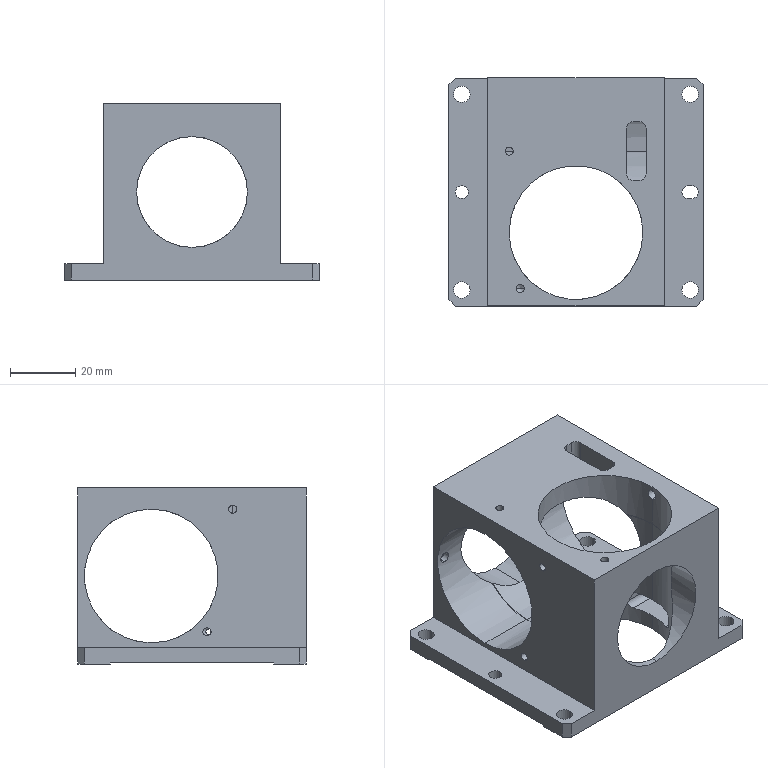NC program | NX | posted with a generic post | part box 78 x 70 x 54 mm
Lines 34 to 1029 of 5040:
(ZLEVEL_PROFILE , TOOL : D20)
N60 T02 M6
N62 G54
N64 G17 G0 G90 X-17.552 Y-45.1 B0. C0. S9500 M3
N66 G43 Z30. H2
N68 Z1.5
N70 G94 G1 X-37.779 Z0.44 F1000.
N72 X-39.872 Y-44.714 Z0.328
N74 X-41.838 Y-43.9 Z0.217
N76 X-43.591 Y-42.693 Z0.105
N78 X-46.693 Y-39.591 Z-0.125
N80 X-47.9 Y-37.838 Z-0.236
N82 X-48.714 Y-35.872 Z-0.348
N84 X-49.1 Y-33.779 Z-0.459
N86 Y-33. Z-0.5
N88 Y33. F3000.
N90 G2 X-46.142 Y40.142 R10.1
N92 G1 X-44.142 Y42.142
N94 G2 X-37. Y45.1 R10.1
N96 G1 X37.
N98 G2 X44.142 Y42.142 R10.1
N100 G1 X46.142 Y40.142
N102 G2 X49.1 Y33. R10.1
N104 G1 Y-33.
N106 G2 X46.142 Y-40.142 R10.1
N108 G1 X44.142 Y-42.142
N110 G2 X37. Y-45.1 R10.1
N112 G1 X-37.
N114 G2 X-44.142 Y-42.142 R10.1
N116 G1 X-46.142 Y-40.142
N118 G2 X-49.1 Y-33. R10.1
N120 G1 Y-4.355 Z-1.
N122 Y33.
N124 G2 X-46.142 Y40.142 R10.1
N126 G1 X-44.142 Y42.142
N128 G2 X-37. Y45.1 R10.1
N130 G1 X37.
N132 G2 X44.142 Y42.142 R10.1
N134 G1 X46.142 Y40.142
N136 G2 X49.1 Y33. R10.1
N138 G1 Y-33.
N140 G2 X46.142 Y-40.142 R10.1
N142 G1 X44.142 Y-42.142
N144 G2 X37. Y-45.1 R10.1
N146 G1 X-37.
N148 G2 X-44.142 Y-42.142 R10.1
N150 G1 X-46.142 Y-40.142
N152 G2 X-49.1 Y-33. R10.1
N154 G1 Y-4.355 Z-1.5
N156 Y33.
N158 G2 X-46.142 Y40.142 R10.1
N160 G1 X-44.142 Y42.142
N162 G2 X-37. Y45.1 R10.1
N164 G1 X37.
N166 G2 X44.142 Y42.142 R10.1
N168 G1 X46.142 Y40.142
N170 G2 X49.1 Y33. R10.1
N172 G1 Y-33.
N174 G2 X46.142 Y-40.142 R10.1
N176 G1 X44.142 Y-42.142
N178 G2 X37. Y-45.1 R10.1
N180 G1 X-37.
N182 G2 X-44.142 Y-42.142 R10.1
N184 G1 X-46.142 Y-40.142
N186 G2 X-49.1 Y-33. R10.1
N188 G1 Y-4.355 Z-2.
N190 Y33.
N192 G2 X-46.142 Y40.142 R10.1
N194 G1 X-44.142 Y42.142
N196 G2 X-37. Y45.1 R10.1
N198 G1 X37.
N200 G2 X44.142 Y42.142 R10.1
N202 G1 X46.142 Y40.142
N204 G2 X49.1 Y33. R10.1
N206 G1 Y-33.
N208 G2 X46.142 Y-40.142 R10.1
N210 G1 X44.142 Y-42.142
N212 G2 X37. Y-45.1 R10.1
N214 G1 X-37.
N216 G2 X-44.142 Y-42.142 R10.1
N218 G1 X-46.142 Y-40.142
N220 G2 X-49.1 Y-33. R10.1
N222 G1 Y-4.355 Z-2.5
N224 Y33.
N226 G2 X-46.142 Y40.142 R10.1
N228 G1 X-44.142 Y42.142
N230 G2 X-37. Y45.1 R10.1
N232 G1 X37.
N234 G2 X44.142 Y42.142 R10.1
N236 G1 X46.142 Y40.142
N238 G2 X49.1 Y33. R10.1
N240 G1 Y-33.
N242 G2 X46.142 Y-40.142 R10.1
N244 G1 X44.142 Y-42.142
N246 G2 X37. Y-45.1 R10.1
N248 G1 X-37.
N250 G2 X-44.142 Y-42.142 R10.1
N252 G1 X-46.142 Y-40.142
N254 G2 X-49.1 Y-33. R10.1
N256 G1 Y-4.355 Z-3.
N258 Y33.
N260 G2 X-46.142 Y40.142 R10.1
N262 G1 X-44.142 Y42.142
N264 G2 X-37. Y45.1 R10.1
N266 G1 X37.
N268 G2 X44.142 Y42.142 R10.1
N270 G1 X46.142 Y40.142
N272 G2 X49.1 Y33. R10.1
N274 G1 Y-33.
N276 G2 X46.142 Y-40.142 R10.1
N278 G1 X44.142 Y-42.142
N280 G2 X37. Y-45.1 R10.1
N282 G1 X-37.
N284 G2 X-44.142 Y-42.142 R10.1
N286 G1 X-46.142 Y-40.142
N288 G2 X-49.1 Y-33. R10.1
N290 G1 Y-4.355 Z-3.5
N292 Y33.
N294 G2 X-46.142 Y40.142 R10.1
N296 G1 X-44.142 Y42.142
N298 G2 X-37. Y45.1 R10.1
N300 G1 X37.
N302 G2 X44.142 Y42.142 R10.1
N304 G1 X46.142 Y40.142
N306 G2 X49.1 Y33. R10.1
N308 G1 Y-33.
N310 G2 X46.142 Y-40.142 R10.1
N312 G1 X44.142 Y-42.142
N314 G2 X37. Y-45.1 R10.1
N316 G1 X-37.
N318 G2 X-44.142 Y-42.142 R10.1
N320 G1 X-46.142 Y-40.142
N322 G2 X-49.1 Y-33. R10.1
N324 G1 Y-4.355 Z-4.
N326 Y33.
N328 G2 X-46.142 Y40.142 R10.1
N330 G1 X-44.142 Y42.142
N332 G2 X-37. Y45.1 R10.1
N334 G1 X37.
N336 G2 X44.142 Y42.142 R10.1
N338 G1 X46.142 Y40.142
N340 G2 X49.1 Y33. R10.1
N342 G1 Y-33.
N344 G2 X46.142 Y-40.142 R10.1
N346 G1 X44.142 Y-42.142
N348 G2 X37. Y-45.1 R10.1
N350 G1 X-37.
N352 G2 X-44.142 Y-42.142 R10.1
N354 G1 X-46.142 Y-40.142
N356 G2 X-49.1 Y-33. R10.1
N358 G1 Y-4.355 Z-4.5
N360 Y33.
N362 G2 X-46.142 Y40.142 R10.1
N364 G1 X-44.142 Y42.142
N366 G2 X-37. Y45.1 R10.1
N368 G1 X37.
N370 G2 X44.142 Y42.142 R10.1
N372 G1 X46.142 Y40.142
N374 G2 X49.1 Y33. R10.1
N376 G1 Y-33.
N378 G2 X46.142 Y-40.142 R10.1
N380 G1 X44.142 Y-42.142
N382 G2 X37. Y-45.1 R10.1
N384 G1 X-37.
N386 G2 X-44.142 Y-42.142 R10.1
N388 G1 X-46.142 Y-40.142
N390 G2 X-49.1 Y-33. R10.1
N392 G1 Y-4.355 Z-5.
N394 Y33.
N396 G2 X-46.142 Y40.142 R10.1
N398 G1 X-44.142 Y42.142
N400 G2 X-37. Y45.1 R10.1
N402 G1 X37.
N404 G2 X44.142 Y42.142 R10.1
N406 G1 X46.142 Y40.142
N408 G2 X49.1 Y33. R10.1
N410 G1 Y-33.
N412 G2 X46.142 Y-40.142 R10.1
N414 G1 X44.142 Y-42.142
N416 G2 X37. Y-45.1 R10.1
N418 G1 X-37.
N420 G2 X-44.142 Y-42.142 R10.1
N422 G1 X-46.142 Y-40.142
N424 G2 X-49.1 Y-33. R10.1
N426 G1 Y-4.355 Z-5.5
N428 Y33.
N430 G2 X-46.142 Y40.142 R10.1
N432 G1 X-44.142 Y42.142
N434 G2 X-37. Y45.1 R10.1
N436 G1 X37.
N438 G2 X44.142 Y42.142 R10.1
N440 G1 X46.142 Y40.142
N442 G2 X49.1 Y33. R10.1
N444 G1 Y-33.
N446 G2 X46.142 Y-40.142 R10.1
N448 G1 X44.142 Y-42.142
N450 G2 X37. Y-45.1 R10.1
N452 G1 X-37.
N454 G2 X-44.142 Y-42.142 R10.1
N456 G1 X-46.142 Y-40.142
N458 G2 X-49.1 Y-33. R10.1
N460 G1 Y-4.355 Z-6.
N462 Y33.
N464 G2 X-46.142 Y40.142 R10.1
N466 G1 X-44.142 Y42.142
N468 G2 X-37. Y45.1 R10.1
N470 G1 X37.
N472 G2 X44.142 Y42.142 R10.1
N474 G1 X46.142 Y40.142
N476 G2 X49.1 Y33. R10.1
N478 G1 Y-33.
N480 G2 X46.142 Y-40.142 R10.1
N482 G1 X44.142 Y-42.142
N484 G2 X37. Y-45.1 R10.1
N486 G1 X-37.
N488 G2 X-44.142 Y-42.142 R10.1
N490 G1 X-46.142 Y-40.142
N492 G2 X-49.1 Y-33. R10.1
N494 G1 Y-4.355 Z-6.5
N496 Y33.
N498 G2 X-46.142 Y40.142 R10.1
N500 G1 X-44.142 Y42.142
N502 G2 X-37. Y45.1 R10.1
N504 G1 X37.
N506 G2 X44.142 Y42.142 R10.1
N508 G1 X46.142 Y40.142
N510 G2 X49.1 Y33. R10.1
N512 G1 Y-33.
N514 G2 X46.142 Y-40.142 R10.1
N516 G1 X44.142 Y-42.142
N518 G2 X37. Y-45.1 R10.1
N520 G1 X-37.
N522 G2 X-44.142 Y-42.142 R10.1
N524 G1 X-46.142 Y-40.142
N526 G2 X-49.1 Y-33. R10.1
N528 G1 Y-4.355 Z-7.
N530 Y33.
N532 G2 X-46.142 Y40.142 R10.1
N534 G1 X-44.142 Y42.142
N536 G2 X-37. Y45.1 R10.1
N538 G1 X37.
N540 G2 X44.142 Y42.142 R10.1
N542 G1 X46.142 Y40.142
N544 G2 X49.1 Y33. R10.1
N546 G1 Y-33.
N548 G2 X46.142 Y-40.142 R10.1
N550 G1 X44.142 Y-42.142
N552 G2 X37. Y-45.1 R10.1
N554 G1 X-37.
N556 G2 X-44.142 Y-42.142 R10.1
N558 G1 X-46.142 Y-40.142
N560 G2 X-49.1 Y-33. R10.1
N562 G1 Y-4.355 Z-7.5
N564 Y33.
N566 G2 X-46.142 Y40.142 R10.1
N568 G1 X-44.142 Y42.142
N570 G2 X-37. Y45.1 R10.1
N572 G1 X37.
N574 G2 X44.142 Y42.142 R10.1
N576 G1 X46.142 Y40.142
N578 G2 X49.1 Y33. R10.1
N580 G1 Y-33.
N582 G2 X46.142 Y-40.142 R10.1
N584 G1 X44.142 Y-42.142
N586 G2 X37. Y-45.1 R10.1
N588 G1 X-37.
N590 G2 X-44.142 Y-42.142 R10.1
N592 G1 X-46.142 Y-40.142
N594 G2 X-49.1 Y-33. R10.1
N596 G1 Y-4.355 Z-8.
N598 Y33.
N600 G2 X-46.142 Y40.142 R10.1
N602 G1 X-44.142 Y42.142
N604 G2 X-37. Y45.1 R10.1
N606 G1 X37.
N608 G2 X44.142 Y42.142 R10.1
N610 G1 X46.142 Y40.142
N612 G2 X49.1 Y33. R10.1
N614 G1 Y-33.
N616 G2 X46.142 Y-40.142 R10.1
N618 G1 X44.142 Y-42.142
N620 G2 X37. Y-45.1 R10.1
N622 G1 X-37.
N624 G2 X-44.142 Y-42.142 R10.1
N626 G1 X-46.142 Y-40.142
N628 G2 X-49.1 Y-33. R10.1
N630 G1 Y-4.355 Z-8.5
N632 Y33.
N634 G2 X-46.142 Y40.142 R10.1
N636 G1 X-44.142 Y42.142
N638 G2 X-37. Y45.1 R10.1
N640 G1 X37.
N642 G2 X44.142 Y42.142 R10.1
N644 G1 X46.142 Y40.142
N646 G2 X49.1 Y33. R10.1
N648 G1 Y-33.
N650 G2 X46.142 Y-40.142 R10.1
N652 G1 X44.142 Y-42.142
N654 G2 X37. Y-45.1 R10.1
N656 G1 X-37.
N658 G2 X-44.142 Y-42.142 R10.1
N660 G1 X-46.142 Y-40.142
N662 G2 X-49.1 Y-33. R10.1
N664 G1 Y-4.355 Z-9.
N666 Y33.
N668 G2 X-46.142 Y40.142 R10.1
N670 G1 X-44.142 Y42.142
N672 G2 X-37. Y45.1 R10.1
N674 G1 X37.
N676 G2 X44.142 Y42.142 R10.1
N678 G1 X46.142 Y40.142
N680 G2 X49.1 Y33. R10.1
N682 G1 Y-33.
N684 G2 X46.142 Y-40.142 R10.1
N686 G1 X44.142 Y-42.142
N688 G2 X37. Y-45.1 R10.1
N690 G1 X-37.
N692 G2 X-44.142 Y-42.142 R10.1
N694 G1 X-46.142 Y-40.142
N696 G2 X-49.1 Y-33. R10.1
N698 G1 Y-4.355 Z-9.5
N700 Y33.
N702 G2 X-46.142 Y40.142 R10.1
N704 G1 X-44.142 Y42.142
N706 G2 X-37. Y45.1 R10.1
N708 G1 X37.
N710 G2 X44.142 Y42.142 R10.1
N712 G1 X46.142 Y40.142
N714 G2 X49.1 Y33. R10.1
N716 G1 Y-33.
N718 G2 X46.142 Y-40.142 R10.1
N720 G1 X44.142 Y-42.142
N722 G2 X37. Y-45.1 R10.1
N724 G1 X-37.
N726 G2 X-44.142 Y-42.142 R10.1
N728 G1 X-46.142 Y-40.142
N730 G2 X-49.1 Y-33. R10.1
N732 G1 Y-4.355 Z-10.
N734 Y33.
N736 G2 X-46.142 Y40.142 R10.1
N738 G1 X-44.142 Y42.142
N740 G2 X-37. Y45.1 R10.1
N742 G1 X37.
N744 G2 X44.142 Y42.142 R10.1
N746 G1 X46.142 Y40.142
N748 G2 X49.1 Y33. R10.1
N750 G1 Y-33.
N752 G2 X46.142 Y-40.142 R10.1
N754 G1 X44.142 Y-42.142
N756 G2 X37. Y-45.1 R10.1
N758 G1 X-37.
N760 G2 X-44.142 Y-42.142 R10.1
N762 G1 X-46.142 Y-40.142
N764 G2 X-49.1 Y-33. R10.1
N766 G1 Y-4.355 Z-10.5
N768 Y33.
N770 G2 X-46.142 Y40.142 R10.1
N772 G1 X-44.142 Y42.142
N774 G2 X-37. Y45.1 R10.1
N776 G1 X37.
N778 G2 X44.142 Y42.142 R10.1
N780 G1 X46.142 Y40.142
N782 G2 X49.1 Y33. R10.1
N784 G1 Y-33.
N786 G2 X46.142 Y-40.142 R10.1
N788 G1 X44.142 Y-42.142
N790 G2 X37. Y-45.1 R10.1
N792 G1 X-37.
N794 G2 X-44.142 Y-42.142 R10.1
N796 G1 X-46.142 Y-40.142
N798 G2 X-49.1 Y-33. R10.1
N800 G1 Y-4.355 Z-11.
N802 Y33.
N804 G2 X-46.142 Y40.142 R10.1
N806 G1 X-44.142 Y42.142
N808 G2 X-37. Y45.1 R10.1
N810 G1 X37.
N812 G2 X44.142 Y42.142 R10.1
N814 G1 X46.142 Y40.142
N816 G2 X49.1 Y33. R10.1
N818 G1 Y-33.
N820 G2 X46.142 Y-40.142 R10.1
N822 G1 X44.142 Y-42.142
N824 G2 X37. Y-45.1 R10.1
N826 G1 X-37.
N828 G2 X-44.142 Y-42.142 R10.1
N830 G1 X-46.142 Y-40.142
N832 G2 X-49.1 Y-33. R10.1
N834 G1 Y-4.355 Z-11.5
N836 Y33.
N838 G2 X-46.142 Y40.142 R10.1
N840 G1 X-44.142 Y42.142
N842 G2 X-37. Y45.1 R10.1
N844 G1 X37.
N846 G2 X44.142 Y42.142 R10.1
N848 G1 X46.142 Y40.142
N850 G2 X49.1 Y33. R10.1
N852 G1 Y-33.
N854 G2 X46.142 Y-40.142 R10.1
N856 G1 X44.142 Y-42.142
N858 G2 X37. Y-45.1 R10.1
N860 G1 X-37.
N862 G2 X-44.142 Y-42.142 R10.1
N864 G1 X-46.142 Y-40.142
N866 G2 X-49.1 Y-33. R10.1
N868 G1 Y-4.355 Z-12.
N870 Y33.
N872 G2 X-46.142 Y40.142 R10.1
N874 G1 X-44.142 Y42.142
N876 G2 X-37. Y45.1 R10.1
N878 G1 X37.
N880 G2 X44.142 Y42.142 R10.1
N882 G1 X46.142 Y40.142
N884 G2 X49.1 Y33. R10.1
N886 G1 Y-33.
N888 G2 X46.142 Y-40.142 R10.1
N890 G1 X44.142 Y-42.142
N892 G2 X37. Y-45.1 R10.1
N894 G1 X-37.
N896 G2 X-44.142 Y-42.142 R10.1
N898 G1 X-46.142 Y-40.142
N900 G2 X-49.1 Y-33. R10.1
N902 G1 Y-4.355 Z-12.5
N904 Y33.
N906 G2 X-46.142 Y40.142 R10.1
N908 G1 X-44.142 Y42.142
N910 G2 X-37. Y45.1 R10.1
N912 G1 X37.
N914 G2 X44.142 Y42.142 R10.1
N916 G1 X46.142 Y40.142
N918 G2 X49.1 Y33. R10.1
N920 G1 Y-33.
N922 G2 X46.142 Y-40.142 R10.1
N924 G1 X44.142 Y-42.142
N926 G2 X37. Y-45.1 R10.1
N928 G1 X-37.
N930 G2 X-44.142 Y-42.142 R10.1
N932 G1 X-46.142 Y-40.142
N934 G2 X-49.1 Y-33. R10.1
N936 G1 Y-4.355 Z-13.
N938 Y33.
N940 G2 X-46.142 Y40.142 R10.1
N942 G1 X-44.142 Y42.142
N944 G2 X-37. Y45.1 R10.1
N946 G1 X37.
N948 G2 X44.142 Y42.142 R10.1
N950 G1 X46.142 Y40.142
N952 G2 X49.1 Y33. R10.1
N954 G1 Y-33.
N956 G2 X46.142 Y-40.142 R10.1
N958 G1 X44.142 Y-42.142
N960 G2 X37. Y-45.1 R10.1
N962 G1 X-37.
N964 G2 X-44.142 Y-42.142 R10.1
N966 G1 X-46.142 Y-40.142
N968 G2 X-49.1 Y-33. R10.1
N970 G1 Y-4.355 Z-13.5
N972 Y33.
N974 G2 X-46.142 Y40.142 R10.1
N976 G1 X-44.142 Y42.142
N978 G2 X-37. Y45.1 R10.1
N980 G1 X37.
N982 G2 X44.142 Y42.142 R10.1
N984 G1 X46.142 Y40.142
N986 G2 X49.1 Y33. R10.1
N988 G1 Y-33.
N990 G2 X46.142 Y-40.142 R10.1
N992 G1 X44.142 Y-42.142
N994 G2 X37. Y-45.1 R10.1
N996 G1 X-37.
N998 G2 X-44.142 Y-42.142 R10.1
N1000 G1 X-46.142 Y-40.142
N1002 G2 X-49.1 Y-33. R10.1
N1004 G1 Y-4.355 Z-14.
N1006 Y33.
N1008 G2 X-46.142 Y40.142 R10.1
N1010 G1 X-44.142 Y42.142
N1012 G2 X-37. Y45.1 R10.1
N1014 G1 X37.
N1016 G2 X44.142 Y42.142 R10.1
N1018 G1 X46.142 Y40.142
N1020 G2 X49.1 Y33. R10.1
N1022 G1 Y-33.
N1024 G2 X46.142 Y-40.142 R10.1
N1026 G1 X44.142 Y-42.142
N1028 G2 X37. Y-45.1 R10.1
N1030 G1 X-37.
N1032 G2 X-44.142 Y-42.142 R10.1
N1034 G1 X-46.142 Y-40.142
N1036 G2 X-49.1 Y-33. R10.1
N1038 G1 Y-4.355 Z-14.5
N1040 Y33.
N1042 G2 X-46.142 Y40.142 R10.1
N1044 G1 X-44.142 Y42.142
N1046 G2 X-37. Y45.1 R10.1
N1048 G1 X37.
N1050 G2 X44.142 Y42.142 R10.1
N1052 G1 X46.142 Y40.142
N1054 G2 X49.1 Y33. R10.1
N1056 G1 Y-33.
N1058 G2 X46.142 Y-40.142 R10.1
N1060 G1 X44.142 Y-42.142
N1062 G2 X37. Y-45.1 R10.1
N1064 G1 X-37.
N1066 G2 X-44.142 Y-42.142 R10.1
N1068 G1 X-46.142 Y-40.142
N1070 G2 X-49.1 Y-33. R10.1
N1072 G1 Y-4.355 Z-15.
N1074 Y33.
N1076 G2 X-46.142 Y40.142 R10.1
N1078 G1 X-44.142 Y42.142
N1080 G2 X-37. Y45.1 R10.1
N1082 G1 X37.
N1084 G2 X44.142 Y42.142 R10.1
N1086 G1 X46.142 Y40.142
N1088 G2 X49.1 Y33. R10.1
N1090 G1 Y-33.
N1092 G2 X46.142 Y-40.142 R10.1
N1094 G1 X44.142 Y-42.142
N1096 G2 X37. Y-45.1 R10.1
N1098 G1 X-37.
N1100 G2 X-44.142 Y-42.142 R10.1
N1102 G1 X-46.142 Y-40.142
N1104 G2 X-49.1 Y-33. R10.1
N1106 G1 Y-4.355 Z-15.5
N1108 Y33.
N1110 G2 X-46.142 Y40.142 R10.1
N1112 G1 X-44.142 Y42.142
N1114 G2 X-37. Y45.1 R10.1
N1116 G1 X37.
N1118 G2 X44.142 Y42.142 R10.1
N1120 G1 X46.142 Y40.142
N1122 G2 X49.1 Y33. R10.1
N1124 G1 Y-33.
N1126 G2 X46.142 Y-40.142 R10.1
N1128 G1 X44.142 Y-42.142
N1130 G2 X37. Y-45.1 R10.1
N1132 G1 X-37.
N1134 G2 X-44.142 Y-42.142 R10.1
N1136 G1 X-46.142 Y-40.142
N1138 G2 X-49.1 Y-33. R10.1
N1140 G1 Y-4.355 Z-16.
N1142 Y33.
N1144 G2 X-46.142 Y40.142 R10.1
N1146 G1 X-44.142 Y42.142
N1148 G2 X-37. Y45.1 R10.1
N1150 G1 X37.
N1152 G2 X44.142 Y42.142 R10.1
N1154 G1 X46.142 Y40.142
N1156 G2 X49.1 Y33. R10.1
N1158 G1 Y-33.
N1160 G2 X46.142 Y-40.142 R10.1
N1162 G1 X44.142 Y-42.142
N1164 G2 X37. Y-45.1 R10.1
N1166 G1 X-37.
N1168 G2 X-44.142 Y-42.142 R10.1
N1170 G1 X-46.142 Y-40.142
N1172 G2 X-49.1 Y-33. R10.1
N1174 G1 Y-4.355 Z-16.5
N1176 Y33.
N1178 G2 X-46.142 Y40.142 R10.1
N1180 G1 X-44.142 Y42.142
N1182 G2 X-37. Y45.1 R10.1
N1184 G1 X37.
N1186 G2 X44.142 Y42.142 R10.1
N1188 G1 X46.142 Y40.142
N1190 G2 X49.1 Y33. R10.1
N1192 G1 Y-33.
N1194 G2 X46.142 Y-40.142 R10.1
N1196 G1 X44.142 Y-42.142
N1198 G2 X37. Y-45.1 R10.1
N1200 G1 X-37.
N1202 G2 X-44.142 Y-42.142 R10.1
N1204 G1 X-46.142 Y-40.142
N1206 G2 X-49.1 Y-33. R10.1
N1208 G1 Y-4.355 Z-17.
N1210 Y33.
N1212 G2 X-46.142 Y40.142 R10.1
N1214 G1 X-44.142 Y42.142
N1216 G2 X-37. Y45.1 R10.1
N1218 G1 X37.
N1220 G2 X44.142 Y42.142 R10.1
N1222 G1 X46.142 Y40.142
N1224 G2 X49.1 Y33. R10.1
N1226 G1 Y-33.
N1228 G2 X46.142 Y-40.142 R10.1
N1230 G1 X44.142 Y-42.142
N1232 G2 X37. Y-45.1 R10.1
N1234 G1 X-37.
N1236 G2 X-44.142 Y-42.142 R10.1
N1238 G1 X-46.142 Y-40.142
N1240 G2 X-49.1 Y-33. R10.1
N1242 G1 Y-4.355 Z-17.5
N1244 Y33.
N1246 G2 X-46.142 Y40.142 R10.1
N1248 G1 X-44.142 Y42.142
N1250 G2 X-37. Y45.1 R10.1
N1252 G1 X37.
N1254 G2 X44.142 Y42.142 R10.1
N1256 G1 X46.142 Y40.142
N1258 G2 X49.1 Y33. R10.1
N1260 G1 Y-33.
N1262 G2 X46.142 Y-40.142 R10.1
N1264 G1 X44.142 Y-42.142
N1266 G2 X37. Y-45.1 R10.1
N1268 G1 X-37.
N1270 G2 X-44.142 Y-42.142 R10.1
N1272 G1 X-46.142 Y-40.142
N1274 G2 X-49.1 Y-33. R10.1
N1276 G1 Y-4.355 Z-18.
N1278 Y33.
N1280 G2 X-46.142 Y40.142 R10.1
N1282 G1 X-44.142 Y42.142
N1284 G2 X-37. Y45.1 R10.1
N1286 G1 X37.
N1288 G2 X44.142 Y42.142 R10.1
N1290 G1 X46.142 Y40.142
N1292 G2 X49.1 Y33. R10.1
N1294 G1 Y-33.
N1296 G2 X46.142 Y-40.142 R10.1
N1298 G1 X44.142 Y-42.142
N1300 G2 X37. Y-45.1 R10.1
N1302 G1 X-37.
N1304 G2 X-44.142 Y-42.142 R10.1
N1306 G1 X-46.142 Y-40.142
N1308 G2 X-49.1 Y-33. R10.1
N1310 G1 Y-4.355 Z-18.5
N1312 Y33.
N1314 G2 X-46.142 Y40.142 R10.1
N1316 G1 X-44.142 Y42.142
N1318 G2 X-37. Y45.1 R10.1
N1320 G1 X37.
N1322 G2 X44.142 Y42.142 R10.1
N1324 G1 X46.142 Y40.142
N1326 G2 X49.1 Y33. R10.1
N1328 G1 Y-33.
N1330 G2 X46.142 Y-40.142 R10.1
N1332 G1 X44.142 Y-42.142
N1334 G2 X37. Y-45.1 R10.1
N1336 G1 X-37.
N1338 G2 X-44.142 Y-42.142 R10.1
N1340 G1 X-46.142 Y-40.142
N1342 G2 X-49.1 Y-33. R10.1
N1344 G1 Y-4.355 Z-19.
N1346 Y33.
N1348 G2 X-46.142 Y40.142 R10.1
N1350 G1 X-44.142 Y42.142
N1352 G2 X-37. Y45.1 R10.1
N1354 G1 X37.
N1356 G2 X44.142 Y42.142 R10.1
N1358 G1 X46.142 Y40.142
N1360 G2 X49.1 Y33. R10.1
N1362 G1 Y-33.
N1364 G2 X46.142 Y-40.142 R10.1
N1366 G1 X44.142 Y-42.142
N1368 G2 X37. Y-45.1 R10.1
N1370 G1 X-37.
N1372 G2 X-44.142 Y-42.142 R10.1
N1374 G1 X-46.142 Y-40.142
N1376 G2 X-49.1 Y-33. R10.1
N1378 G1 Y-4.355 Z-19.5
N1380 Y33.
N1382 G2 X-46.142 Y40.142 R10.1
N1384 G1 X-44.142 Y42.142
N1386 G2 X-37. Y45.1 R10.1
N1388 G1 X37.
N1390 G2 X44.142 Y42.142 R10.1
N1392 G1 X46.142 Y40.142
N1394 G2 X49.1 Y33. R10.1
N1396 G1 Y-33.
N1398 G2 X46.142 Y-40.142 R10.1
N1400 G1 X44.142 Y-42.142
N1402 G2 X37. Y-45.1 R10.1
N1404 G1 X-37.
N1406 G2 X-44.142 Y-42.142 R10.1
N1408 G1 X-46.142 Y-40.142
N1410 G2 X-49.1 Y-33. R10.1
N1412 G1 Y-4.355 Z-20.
N1414 Y33.
N1416 G2 X-46.142 Y40.142 R10.1
N1418 G1 X-44.142 Y42.142
N1420 G2 X-37. Y45.1 R10.1
N1422 G1 X37.
N1424 G2 X44.142 Y42.142 R10.1
N1426 G1 X46.142 Y40.142
N1428 G2 X49.1 Y33. R10.1
N1430 G1 Y-33.
N1432 G2 X46.142 Y-40.142 R10.1
N1434 G1 X44.142 Y-42.142
N1436 G2 X37. Y-45.1 R10.1
N1438 G1 X-37.
N1440 G2 X-44.142 Y-42.142 R10.1
N1442 G1 X-46.142 Y-40.142
N1444 G2 X-49.1 Y-33. R10.1
N1446 G1 Y-4.355 Z-20.5
N1448 Y33.
N1450 G2 X-46.142 Y40.142 R10.1
N1452 G1 X-44.142 Y42.142
N1454 G2 X-37. Y45.1 R10.1
N1456 G1 X37.
N1458 G2 X44.142 Y42.142 R10.1
N1460 G1 X46.142 Y40.142
N1462 G2 X49.1 Y33. R10.1
N1464 G1 Y-33.
N1466 G2 X46.142 Y-40.142 R10.1
N1468 G1 X44.142 Y-42.142
N1470 G2 X37. Y-45.1 R10.1
N1472 G1 X-37.
N1474 G2 X-44.142 Y-42.142 R10.1
N1476 G1 X-46.142 Y-40.142
N1478 G2 X-49.1 Y-33. R10.1
N1480 G1 Y-4.355 Z-21.
N1482 Y33.
N1484 G2 X-46.142 Y40.142 R10.1
N1486 G1 X-44.142 Y42.142
N1488 G2 X-37. Y45.1 R10.1
N1490 G1 X37.
N1492 G2 X44.142 Y42.142 R10.1
N1494 G1 X46.142 Y40.142
N1496 G2 X49.1 Y33. R10.1
N1498 G1 Y-33.
N1500 G2 X46.142 Y-40.142 R10.1
N1502 G1 X44.142 Y-42.142
N1504 G2 X37. Y-45.1 R10.1
N1506 G1 X-37.
N1508 G2 X-44.142 Y-42.142 R10.1
N1510 G1 X-46.142 Y-40.142
N1512 G2 X-49.1 Y-33. R10.1
N1514 G1 Y-4.355 Z-21.5
N1516 Y33.
N1518 G2 X-46.142 Y40.142 R10.1
N1520 G1 X-44.142 Y42.142
N1522 G2 X-37. Y45.1 R10.1
N1524 G1 X37.
N1526 G2 X44.142 Y42.142 R10.1
N1528 G1 X46.142 Y40.142
N1530 G2 X49.1 Y33. R10.1
N1532 G1 Y-33.
N1534 G2 X46.142 Y-40.142 R10.1
N1536 G1 X44.142 Y-42.142
N1538 G2 X37. Y-45.1 R10.1
N1540 G1 X-37.
N1542 G2 X-44.142 Y-42.142 R10.1
N1544 G1 X-46.142 Y-40.142
N1546 G2 X-49.1 Y-33. R10.1
N1548 G1 Y-4.355 Z-22.
N1550 Y33.
N1552 G2 X-46.142 Y40.142 R10.1
N1554 G1 X-44.142 Y42.142
N1556 G2 X-37. Y45.1 R10.1
N1558 G1 X37.
N1560 G2 X44.142 Y42.142 R10.1
N1562 G1 X46.142 Y40.142
N1564 G2 X49.1 Y33. R10.1
N1566 G1 Y-33.
N1568 G2 X46.142 Y-40.142 R10.1
N1570 G1 X44.142 Y-42.142
N1572 G2 X37. Y-45.1 R10.1
N1574 G1 X-37.
N1576 G2 X-44.142 Y-42.142 R10.1
N1578 G1 X-46.142 Y-40.142
N1580 G2 X-49.1 Y-33. R10.1
N1582 G1 Y-4.355 Z-22.5
N1584 Y33.
N1586 G2 X-46.142 Y40.142 R10.1
N1588 G1 X-44.142 Y42.142
N1590 G2 X-37. Y45.1 R10.1
N1592 G1 X37.
N1594 G2 X44.142 Y42.142 R10.1
N1596 G1 X46.142 Y40.142
N1598 G2 X49.1 Y33. R10.1
N1600 G1 Y-33.
N1602 G2 X46.142 Y-40.142 R10.1
N1604 G1 X44.142 Y-42.142
N1606 G2 X37. Y-45.1 R10.1
N1608 G1 X-37.
N1610 G2 X-44.142 Y-42.142 R10.1
N1612 G1 X-46.142 Y-40.142
N1614 G2 X-49.1 Y-33. R10.1
N1616 G1 Y-4.355 Z-23.
N1618 Y33.
N1620 G2 X-46.142 Y40.142 R10.1
N1622 G1 X-44.142 Y42.142
N1624 G2 X-37. Y45.1 R10.1
N1626 G1 X37.
N1628 G2 X44.142 Y42.142 R10.1
N1630 G1 X46.142 Y40.142
N1632 G2 X49.1 Y33. R10.1
N1634 G1 Y-33.
N1636 G2 X46.142 Y-40.142 R10.1
N1638 G1 X44.142 Y-42.142
N1640 G2 X37. Y-45.1 R10.1
N1642 G1 X-37.
N1644 G2 X-44.142 Y-42.142 R10.1
N1646 G1 X-46.142 Y-40.142
N1648 G2 X-49.1 Y-33. R10.1
N1650 G1 Y-4.355 Z-23.5
N1652 Y33.
N1654 G2 X-46.142 Y40.142 R10.1
N1656 G1 X-44.142 Y42.142
N1658 G2 X-37. Y45.1 R10.1
N1660 G1 X37.
N1662 G2 X44.142 Y42.142 R10.1
N1664 G1 X46.142 Y40.142
N1666 G2 X49.1 Y33. R10.1
N1668 G1 Y-33.
N1670 G2 X46.142 Y-40.142 R10.1
N1672 G1 X44.142 Y-42.142
N1674 G2 X37. Y-45.1 R10.1
N1676 G1 X-37.
N1678 G2 X-44.142 Y-42.142 R10.1
N1680 G1 X-46.142 Y-40.142
N1682 G2 X-49.1 Y-33. R10.1
N1684 G1 Y-4.355 Z-24.
N1686 Y33.
N1688 G2 X-46.142 Y40.142 R10.1
N1690 G1 X-44.142 Y42.142
N1692 G2 X-37. Y45.1 R10.1
N1694 G1 X37.
N1696 G2 X44.142 Y42.142 R10.1
N1698 G1 X46.142 Y40.142
N1700 G2 X49.1 Y33. R10.1
N1702 G1 Y-33.
N1704 G2 X46.142 Y-40.142 R10.1
N1706 G1 X44.142 Y-42.142
N1708 G2 X37. Y-45.1 R10.1
N1710 G1 X-37.
N1712 G2 X-44.142 Y-42.142 R10.1
N1714 G1 X-46.142 Y-40.142
N1716 G2 X-49.1 Y-33. R10.1
N1718 G1 Y-4.355 Z-24.5
N1720 Y33.
N1722 G2 X-46.142 Y40.142 R10.1
N1724 G1 X-44.142 Y42.142
N1726 G2 X-37. Y45.1 R10.1
N1728 G1 X37.
N1730 G2 X44.142 Y42.142 R10.1
N1732 G1 X46.142 Y40.142
N1734 G2 X49.1 Y33. R10.1
N1736 G1 Y-33.
N1738 G2 X46.142 Y-40.142 R10.1
N1740 G1 X44.142 Y-42.142
N1742 G2 X37. Y-45.1 R10.1
N1744 G1 X-37.
N1746 G2 X-44.142 Y-42.142 R10.1
N1748 G1 X-46.142 Y-40.142
N1750 G2 X-49.1 Y-33. R10.1
N1752 G1 Y-4.355 Z-25.
N1754 Y33.
N1756 G2 X-46.142 Y40.142 R10.1
N1758 G1 X-44.142 Y42.142
N1760 G2 X-37. Y45.1 R10.1
N1762 G1 X37.
N1764 G2 X44.142 Y42.142 R10.1
N1766 G1 X46.142 Y40.142
N1768 G2 X49.1 Y33. R10.1
N1770 G1 Y-33.
N1772 G2 X46.142 Y-40.142 R10.1
N1774 G1 X44.142 Y-42.142
N1776 G2 X37. Y-45.1 R10.1
N1778 G1 X-37.
N1780 G2 X-44.142 Y-42.142 R10.1
N1782 G1 X-46.142 Y-40.142
N1784 G2 X-49.1 Y-33. R10.1
N1786 G1 Y-4.355 Z-25.5
N1788 Y33.
N1790 G2 X-46.142 Y40.142 R10.1
N1792 G1 X-44.142 Y42.142
N1794 G2 X-37. Y45.1 R10.1
N1796 G1 X37.
N1798 G2 X44.142 Y42.142 R10.1
N1800 G1 X46.142 Y40.142
N1802 G2 X49.1 Y33. R10.1
N1804 G1 Y-33.
N1806 G2 X46.142 Y-40.142 R10.1
N1808 G1 X44.142 Y-42.142
N1810 G2 X37. Y-45.1 R10.1
N1812 G1 X-37.
N1814 G2 X-44.142 Y-42.142 R10.1
N1816 G1 X-46.142 Y-40.142
N1818 G2 X-49.1 Y-33. R10.1
N1820 G1 Y-4.355 Z-26.
N1822 Y33.
N1824 G2 X-46.142 Y40.142 R10.1
N1826 G1 X-44.142 Y42.142
N1828 G2 X-37. Y45.1 R10.1
N1830 G1 X37.
N1832 G2 X44.142 Y42.142 R10.1
N1834 G1 X46.142 Y40.142
N1836 G2 X49.1 Y33. R10.1
N1838 G1 Y-33.
N1840 G2 X46.142 Y-40.142 R10.1
N1842 G1 X44.142 Y-42.142
N1844 G2 X37. Y-45.1 R10.1
N1846 G1 X-37.
N1848 G2 X-44.142 Y-42.142 R10.1
N1850 G1 X-46.142 Y-40.142
N1852 G2 X-49.1 Y-33. R10.1
N1854 G1 Y-4.355 Z-26.5
N1856 Y33.
N1858 G2 X-46.142 Y40.142 R10.1
N1860 G1 X-44.142 Y42.142
N1862 G2 X-37. Y45.1 R10.1
N1864 G1 X37.
N1866 G2 X44.142 Y42.142 R10.1
N1868 G1 X46.142 Y40.142
N1870 G2 X49.1 Y33. R10.1
N1872 G1 Y-33.
N1874 G2 X46.142 Y-40.142 R10.1
N1876 G1 X44.142 Y-42.142
N1878 G2 X37. Y-45.1 R10.1
N1880 G1 X-37.
N1882 G2 X-44.142 Y-42.142 R10.1
N1884 G1 X-46.142 Y-40.142
N1886 G2 X-49.1 Y-33. R10.1
N1888 G1 Y-4.355 Z-27.
N1890 Y33.
N1892 G2 X-46.142 Y40.142 R10.1
N1894 G1 X-44.142 Y42.142
N1896 G2 X-37. Y45.1 R10.1
N1898 G1 X37.
N1900 G2 X44.142 Y42.142 R10.1
N1902 G1 X46.142 Y40.142
N1904 G2 X49.1 Y33. R10.1
N1906 G1 Y-33.
N1908 G2 X46.142 Y-40.142 R10.1
N1910 G1 X44.142 Y-42.142
N1912 G2 X37. Y-45.1 R10.1
N1914 G1 X-37.
N1916 G2 X-44.142 Y-42.142 R10.1
N1918 G1 X-46.142 Y-40.142
N1920 G2 X-49.1 Y-33. R10.1
N1922 G1 Y-4.355 Z-27.5
N1924 Y33.
N1926 G2 X-46.142 Y40.142 R10.1
N1928 G1 X-44.142 Y42.142
N1930 G2 X-37. Y45.1 R10.1
N1932 G1 X37.
N1934 G2 X44.142 Y42.142 R10.1
N1936 G1 X46.142 Y40.142
N1938 G2 X49.1 Y33. R10.1
N1940 G1 Y-33.
N1942 G2 X46.142 Y-40.142 R10.1
N1944 G1 X44.142 Y-42.142
N1946 G2 X37. Y-45.1 R10.1
N1948 G1 X-37.
N1950 G2 X-44.142 Y-42.142 R10.1
N1952 G1 X-46.142 Y-40.142
N1954 G2 X-49.1 Y-33. R10.1
N1956 G1 Y-4.355 Z-28.
N1958 Y33.
N1960 G2 X-46.142 Y40.142 R10.1
N1962 G1 X-44.142 Y42.142
N1964 G2 X-37. Y45.1 R10.1
N1966 G1 X37.
N1968 G2 X44.142 Y42.142 R10.1
N1970 G1 X46.142 Y40.142
N1972 G2 X49.1 Y33. R10.1
N1974 G1 Y-33.
N1976 G2 X46.142 Y-40.142 R10.1
N1978 G1 X44.142 Y-42.142
N1980 G2 X37. Y-45.1 R10.1
N1982 G1 X-37.
N1984 G2 X-44.142 Y-42.142 R10.1
N1986 G1 X-46.142 Y-40.142
N1988 G2 X-49.1 Y-33. R10.1
N1990 G1 Y-4.355 Z-28.5
N1992 Y33.
N1994 G2 X-46.142 Y40.142 R10.1
N1996 G1 X-44.142 Y42.142
N1998 G2 X-37. Y45.1 R10.1
N2000 G1 X37.
N2002 G2 X44.142 Y42.142 R10.1
N2004 G1 X46.142 Y40.142
N2006 G2 X49.1 Y33. R10.1
N2008 G1 Y-33.
N2010 G2 X46.142 Y-40.142 R10.1
N2012 G1 X44.142 Y-42.142
N2014 G2 X37. Y-45.1 R10.1
N2016 G1 X-37.
N2018 G2 X-44.142 Y-42.142 R10.1
N2020 G1 X-46.142 Y-40.142
N2022 G2 X-49.1 Y-33. R10.1
N2024 G1 Y-4.355 Z-29.
N2026 Y33.
N2028 G2 X-46.142 Y40.142 R10.1
N2030 G1 X-44.142 Y42.142
N2032 G2 X-37. Y45.1 R10.1
N2034 G1 X37.
N2036 G2 X44.142 Y42.142 R10.1
N2038 G1 X46.142 Y40.142
N2040 G2 X49.1 Y33. R10.1
N2042 G1 Y-33.
N2044 G2 X46.142 Y-40.142 R10.1